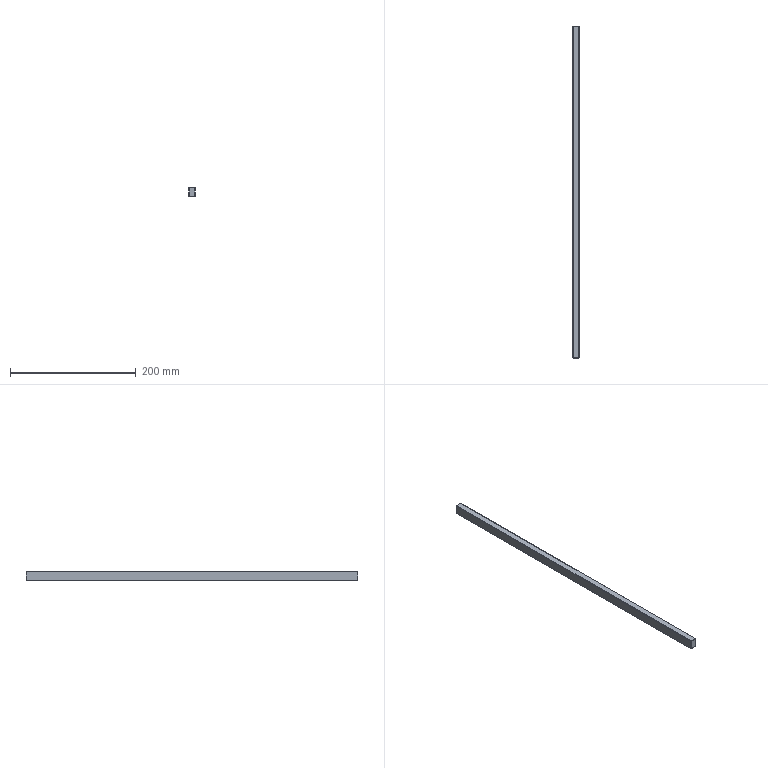Part | STEP file | ESG4 | 1 solid | 26 faces | box 10 x 528 x 15 mm | volume 79081 mm3 | cylinder 12 | spline 8 | plane 6 | commonest cylinder face diameters 1 x12